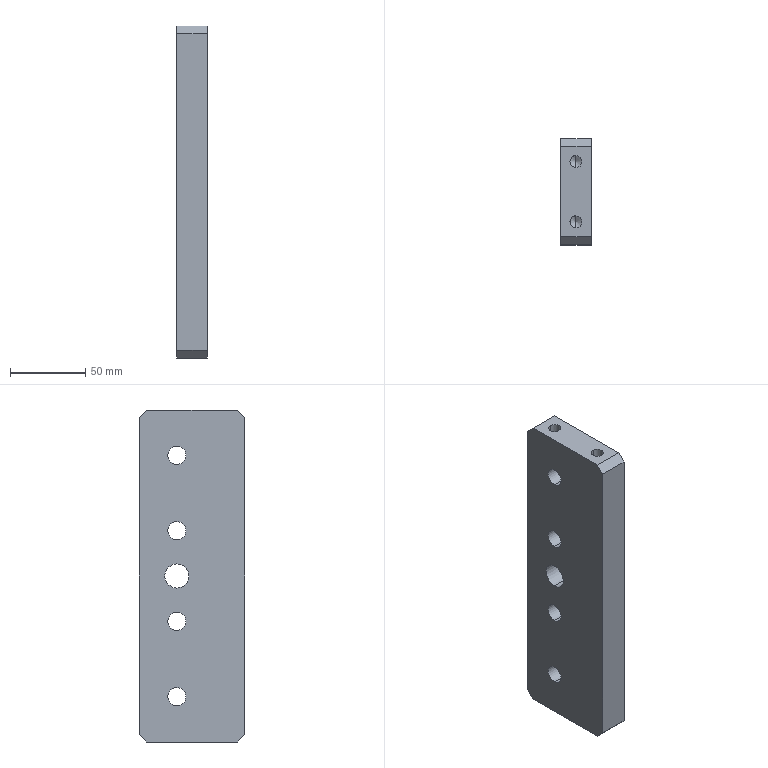Part | STEP file | Positioning_id226_x_t | 1 solid | 34 faces | box 20 x 70 x 220 mm | volume 289829 mm3 | cylinder 18 | plane 12 | cone 4 | commonest cylinder face diameters 8 x8 12 x8 16 x2